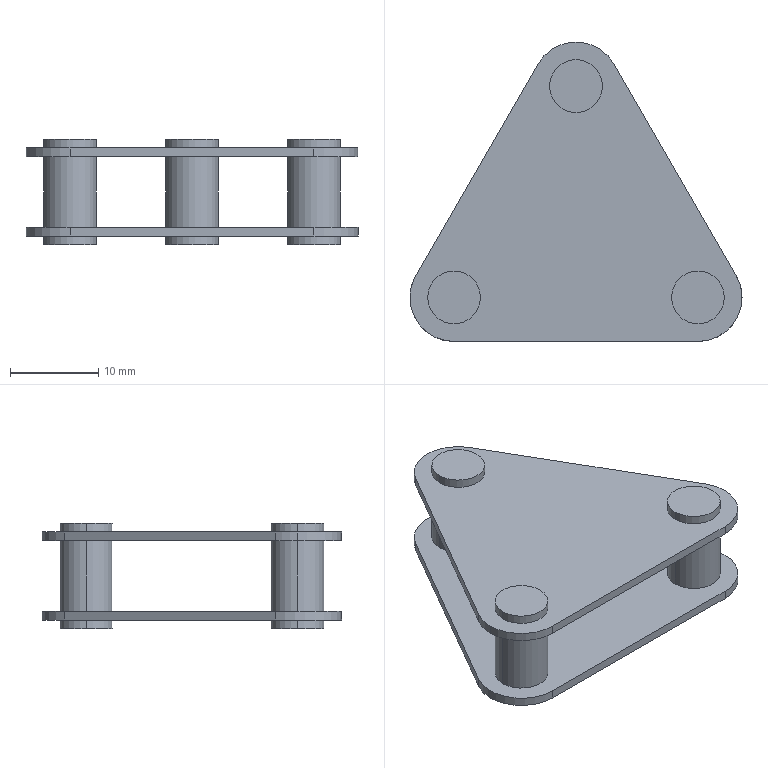Part | SolidWorks | features ICE 2, Extrusion 1, MirrorPattern 1 | 1 solid | 42 faces | box 37.679 x 33.971 x 12 mm | volume 2499 mm3 | cylinder 26 | plane 16 | commonest cylinder face diameters 6 x18 10 x8
STEP:
#1=CARTESIAN_POINT('',(-10.84,-7.99,2.));
#2=VERTEX_POINT('',#1);
#3=CARTESIAN_POINT('',(-16.84,-7.99,2.));
#4=VERTEX_POINT('',#3);
#5=CARTESIAN_POINT('',(-13.84,-7.99,2.));
#6=DIRECTION('',(0.,0.,1.));
#7=DIRECTION('',(1.,0.,0.));
#8=AXIS2_PLACEMENT_3D('',#5,#6,#7);
#9=CIRCLE('',#8,3.);
#10=EDGE_CURVE('',#2,#4,#9,.T.);
#11=ORIENTED_EDGE('',*,*,#10,.F.);
#12=CARTESIAN_POINT('',(-10.84,-7.99,1.));
#13=VERTEX_POINT('',#12);
#14=CARTESIAN_POINT('',(-10.84,-7.99,2.));
#15=DIRECTION('',(0.,0.,-1.));
#16=VECTOR('',#15,1000.);
#17=LINE('',#14,#16);
#18=EDGE_CURVE('',#2,#13,#17,.T.);
#19=ORIENTED_EDGE('',*,*,#18,.T.);
#20=CARTESIAN_POINT('',(-16.84,-7.99,1.));
#21=VERTEX_POINT('',#20);
#22=CARTESIAN_POINT('',(-13.84,-7.99,1.));
#23=DIRECTION('',(0.,0.,1.));
#24=DIRECTION('',(1.,0.,0.));
#25=AXIS2_PLACEMENT_3D('',#22,#23,#24);
#26=CIRCLE('',#25,3.);
#27=EDGE_CURVE('',#13,#21,#26,.T.);
#28=ORIENTED_EDGE('',*,*,#27,.T.);
#29=CARTESIAN_POINT('',(-16.84,-7.99,2.));
#30=DIRECTION('',(0.,0.,-1.));
#31=VECTOR('',#30,1000.);
#32=LINE('',#29,#31);
#33=EDGE_CURVE('',#4,#21,#32,.T.);
#34=ORIENTED_EDGE('',*,*,#33,.F.);
#35=EDGE_LOOP('',(#11,#19,#28,#34));
#36=FACE_OUTER_BOUND('',#35,.T.);
#37=CARTESIAN_POINT('',(-13.84,-7.99,2.));
#38=DIRECTION('',(0.,0.,-1.));
#39=DIRECTION('',(-1.,0.,0.));
#40=AXIS2_PLACEMENT_3D('',#37,#38,#39);
#41=CYLINDRICAL_SURFACE('',#40,3.);
#42=ADVANCED_FACE('',(#36),#41,.T.);
#43=CARTESIAN_POINT('',(16.84,-7.99,2.));
#44=VERTEX_POINT('',#43);
#45=CARTESIAN_POINT('',(10.84,-7.99,2.));
#46=VERTEX_POINT('',#45);
#47=CARTESIAN_POINT('',(13.84,-7.99,2.));
#48=DIRECTION('',(0.,0.,1.));
#49=DIRECTION('',(1.,0.,0.));
#50=AXIS2_PLACEMENT_3D('',#47,#48,#49);
#51=CIRCLE('',#50,3.);
#52=EDGE_CURVE('',#44,#46,#51,.T.);
#53=ORIENTED_EDGE('',*,*,#52,.F.);
#54=CARTESIAN_POINT('',(16.84,-7.99,1.));
#55=VERTEX_POINT('',#54);
#56=CARTESIAN_POINT('',(16.84,-7.99,2.));
#57=DIRECTION('',(0.,0.,-1.));
#58=VECTOR('',#57,1000.);
#59=LINE('',#56,#58);
#60=EDGE_CURVE('',#44,#55,#59,.T.);
#61=ORIENTED_EDGE('',*,*,#60,.T.);
#62=CARTESIAN_POINT('',(10.84,-7.99,1.));
#63=VERTEX_POINT('',#62);
#64=CARTESIAN_POINT('',(13.84,-7.99,1.));
#65=DIRECTION('',(0.,0.,1.));
#66=DIRECTION('',(1.,0.,0.));
#67=AXIS2_PLACEMENT_3D('',#64,#65,#66);
#68=CIRCLE('',#67,3.);
#69=EDGE_CURVE('',#55,#63,#68,.T.);
#70=ORIENTED_EDGE('',*,*,#69,.T.);
#71=CARTESIAN_POINT('',(10.84,-7.99,2.));
#72=DIRECTION('',(0.,0.,-1.));
#73=VECTOR('',#72,1000.);
#74=LINE('',#71,#73);
#75=EDGE_CURVE('',#46,#63,#74,.T.);
#76=ORIENTED_EDGE('',*,*,#75,.F.);
#77=EDGE_LOOP('',(#53,#61,#70,#76));
#78=FACE_OUTER_BOUND('',#77,.T.);
#79=CARTESIAN_POINT('',(13.84,-7.99,2.));
#80=DIRECTION('',(0.,0.,-1.));
#81=DIRECTION('',(-1.,0.,0.));
#82=AXIS2_PLACEMENT_3D('',#79,#80,#81);
#83=CYLINDRICAL_SURFACE('',#82,3.);
#84=ADVANCED_FACE('',(#78),#83,.T.);
#85=CARTESIAN_POINT('',(3.,15.981,2.));
#86=VERTEX_POINT('',#85);
#87=CARTESIAN_POINT('',(-3.,15.981,2.));
#88=VERTEX_POINT('',#87);
#89=CARTESIAN_POINT('',(0.,15.981,2.));
#90=DIRECTION('',(0.,0.,1.));
#91=DIRECTION('',(1.,0.,0.));
#92=AXIS2_PLACEMENT_3D('',#89,#90,#91);
#93=CIRCLE('',#92,3.);
#94=EDGE_CURVE('',#86,#88,#93,.T.);
#95=ORIENTED_EDGE('',*,*,#94,.F.);
#96=CARTESIAN_POINT('',(3.,15.981,1.));
#97=VERTEX_POINT('',#96);
#98=CARTESIAN_POINT('',(3.,15.981,2.));
#99=DIRECTION('',(0.,0.,-1.));
#100=VECTOR('',#99,1000.);
#101=LINE('',#98,#100);
#102=EDGE_CURVE('',#86,#97,#101,.T.);
#103=ORIENTED_EDGE('',*,*,#102,.T.);
#104=CARTESIAN_POINT('',(-3.,15.981,1.));
#105=VERTEX_POINT('',#104);
#106=CARTESIAN_POINT('',(0.,15.981,1.));
#107=DIRECTION('',(0.,0.,1.));
#108=DIRECTION('',(1.,0.,0.));
#109=AXIS2_PLACEMENT_3D('',#106,#107,#108);
#110=CIRCLE('',#109,3.);
#111=EDGE_CURVE('',#97,#105,#110,.T.);
#112=ORIENTED_EDGE('',*,*,#111,.T.);
#113=CARTESIAN_POINT('',(-3.,15.981,2.));
#114=DIRECTION('',(0.,0.,-1.));
#115=VECTOR('',#114,1000.);
#116=LINE('',#113,#115);
#117=EDGE_CURVE('',#88,#105,#116,.T.);
#118=ORIENTED_EDGE('',*,*,#117,.F.);
#119=EDGE_LOOP('',(#95,#103,#112,#118));
#120=FACE_OUTER_BOUND('',#119,.T.);
#121=CARTESIAN_POINT('',(0.,15.981,2.));
#122=DIRECTION('',(0.,0.,-1.));
#123=DIRECTION('',(-1.,0.,0.));
#124=AXIS2_PLACEMENT_3D('',#121,#122,#123);
#125=CYLINDRICAL_SURFACE('',#124,3.);
#126=ADVANCED_FACE('',(#120),#125,.T.);
#127=CARTESIAN_POINT('',(16.84,-7.99,-10.));
#128=VERTEX_POINT('',#127);
#129=CARTESIAN_POINT('',(10.84,-7.99,-10.));
#130=VERTEX_POINT('',#129);
#131=CARTESIAN_POINT('',(13.84,-7.99,-10.));
#132=DIRECTION('',(0.,0.,1.));
#133=DIRECTION('',(1.,0.,0.));
#134=AXIS2_PLACEMENT_3D('',#131,#132,#133);
#135=CIRCLE('',#134,3.);
#136=EDGE_CURVE('',#128,#130,#135,.T.);
#137=ORIENTED_EDGE('',*,*,#136,.T.);
#138=CARTESIAN_POINT('',(10.84,-7.99,-9.));
#139=VERTEX_POINT('',#138);
#140=CARTESIAN_POINT('',(10.84,-7.99,-10.));
#141=DIRECTION('',(0.,0.,1.));
#142=VECTOR('',#141,1000.);
#143=LINE('',#140,#142);
#144=EDGE_CURVE('',#130,#139,#143,.T.);
#145=ORIENTED_EDGE('',*,*,#144,.T.);
#146=CARTESIAN_POINT('',(16.84,-7.99,-9.));
#147=VERTEX_POINT('',#146);
#148=CARTESIAN_POINT('',(13.84,-7.99,-9.));
#149=DIRECTION('',(0.,0.,1.));
#150=DIRECTION('',(-1.,0.,0.));
#151=AXIS2_PLACEMENT_3D('',#148,#149,#150);
#152=CIRCLE('',#151,3.);
#153=EDGE_CURVE('',#147,#139,#152,.T.);
#154=ORIENTED_EDGE('',*,*,#153,.F.);
#155=CARTESIAN_POINT('',(16.84,-7.99,-10.));
#156=DIRECTION('',(0.,0.,1.));
#157=VECTOR('',#156,1000.);
#158=LINE('',#155,#157);
#159=EDGE_CURVE('',#128,#147,#158,.T.);
#160=ORIENTED_EDGE('',*,*,#159,.F.);
#161=EDGE_LOOP('',(#137,#145,#154,#160));
#162=FACE_OUTER_BOUND('',#161,.T.);
#163=CARTESIAN_POINT('',(13.84,-7.99,-10.));
#164=DIRECTION('',(0.,0.,1.));
#165=DIRECTION('',(1.,0.,0.));
#166=AXIS2_PLACEMENT_3D('',#163,#164,#165);
#167=CYLINDRICAL_SURFACE('',#166,3.);
#168=ADVANCED_FACE('',(#162),#167,.T.);
#169=CARTESIAN_POINT('',(-10.84,-7.99,-10.));
#170=VERTEX_POINT('',#169);
#171=CARTESIAN_POINT('',(-16.84,-7.99,-10.));
#172=VERTEX_POINT('',#171);
#173=CARTESIAN_POINT('',(-13.84,-7.99,-10.));
#174=DIRECTION('',(0.,0.,1.));
#175=DIRECTION('',(1.,0.,0.));
#176=AXIS2_PLACEMENT_3D('',#173,#174,#175);
#177=CIRCLE('',#176,3.);
#178=EDGE_CURVE('',#170,#172,#177,.T.);
#179=ORIENTED_EDGE('',*,*,#178,.T.);
#180=CARTESIAN_POINT('',(-16.84,-7.99,-9.));
#181=VERTEX_POINT('',#180);
#182=CARTESIAN_POINT('',(-16.84,-7.99,-10.));
#183=DIRECTION('',(0.,0.,1.));
#184=VECTOR('',#183,1000.);
#185=LINE('',#182,#184);
#186=EDGE_CURVE('',#172,#181,#185,.T.);
#187=ORIENTED_EDGE('',*,*,#186,.T.);
#188=CARTESIAN_POINT('',(-10.84,-7.99,-9.));
#189=VERTEX_POINT('',#188);
#190=CARTESIAN_POINT('',(-13.84,-7.99,-9.));
#191=DIRECTION('',(0.,0.,1.));
#192=DIRECTION('',(-1.,0.,0.));
#193=AXIS2_PLACEMENT_3D('',#190,#191,#192);
#194=CIRCLE('',#193,3.);
#195=EDGE_CURVE('',#189,#181,#194,.T.);
#196=ORIENTED_EDGE('',*,*,#195,.F.);
#197=CARTESIAN_POINT('',(-10.84,-7.99,-10.));
#198=DIRECTION('',(0.,0.,1.));
#199=VECTOR('',#198,1000.);
#200=LINE('',#197,#199);
#201=EDGE_CURVE('',#170,#189,#200,.T.);
#202=ORIENTED_EDGE('',*,*,#201,.F.);
#203=EDGE_LOOP('',(#179,#187,#196,#202));
#204=FACE_OUTER_BOUND('',#203,.T.);
#205=CARTESIAN_POINT('',(-13.84,-7.99,-10.));
#206=DIRECTION('',(0.,0.,1.));
#207=DIRECTION('',(1.,0.,0.));
#208=AXIS2_PLACEMENT_3D('',#205,#206,#207);
#209=CYLINDRICAL_SURFACE('',#208,3.);
#210=ADVANCED_FACE('',(#204),#209,.T.);
#211=CARTESIAN_POINT('',(3.,15.981,-10.));
#212=VERTEX_POINT('',#211);
#213=CARTESIAN_POINT('',(-3.,15.981,-10.));
#214=VERTEX_POINT('',#213);
#215=CARTESIAN_POINT('',(0.,15.981,-10.));
#216=DIRECTION('',(0.,0.,1.));
#217=DIRECTION('',(1.,0.,0.));
#218=AXIS2_PLACEMENT_3D('',#215,#216,#217);
#219=CIRCLE('',#218,3.);
#220=EDGE_CURVE('',#212,#214,#219,.T.);
#221=ORIENTED_EDGE('',*,*,#220,.T.);
#222=CARTESIAN_POINT('',(-3.,15.981,-9.));
#223=VERTEX_POINT('',#222);
#224=CARTESIAN_POINT('',(-3.,15.981,-10.));
#225=DIRECTION('',(0.,0.,1.));
#226=VECTOR('',#225,1000.);
#227=LINE('',#224,#226);
#228=EDGE_CURVE('',#214,#223,#227,.T.);
#229=ORIENTED_EDGE('',*,*,#228,.T.);
#230=CARTESIAN_POINT('',(3.,15.981,-9.));
#231=VERTEX_POINT('',#230);
#232=CARTESIAN_POINT('',(0.,15.981,-9.));
#233=DIRECTION('',(0.,0.,1.));
#234=DIRECTION('',(-1.,0.,0.));
#235=AXIS2_PLACEMENT_3D('',#232,#233,#234);
#236=CIRCLE('',#235,3.);
#237=EDGE_CURVE('',#231,#223,#236,.T.);
#238=ORIENTED_EDGE('',*,*,#237,.F.);
#239=CARTESIAN_POINT('',(3.,15.981,-10.));
#240=DIRECTION('',(0.,0.,1.));
#241=VECTOR('',#240,1000.);
#242=LINE('',#239,#241);
#243=EDGE_CURVE('',#212,#231,#242,.T.);
#244=ORIENTED_EDGE('',*,*,#243,.F.);
#245=EDGE_LOOP('',(#221,#229,#238,#244));
#246=FACE_OUTER_BOUND('',#245,.T.);
#247=CARTESIAN_POINT('',(0.,15.981,-10.));
#248=DIRECTION('',(0.,0.,1.));
#249=DIRECTION('',(1.,0.,0.));
#250=AXIS2_PLACEMENT_3D('',#247,#248,#249);
#251=CYLINDRICAL_SURFACE('',#250,3.);
#252=ADVANCED_FACE('',(#246),#251,.T.);
#253=CARTESIAN_POINT('',(13.84,-12.99,-9.));
#254=VERTEX_POINT('',#253);
#255=CARTESIAN_POINT('',(18.84,-7.99,-9.));
#256=VERTEX_POINT('',#255);
#257=CARTESIAN_POINT('',(13.84,-7.99,-9.));
#258=DIRECTION('',(0.,0.,1.));
#259=DIRECTION('',(1.,0.,0.));
#260=AXIS2_PLACEMENT_3D('',#257,#258,#259);
#261=CIRCLE('',#260,5.);
#262=EDGE_CURVE('',#254,#256,#261,.T.);
#263=ORIENTED_EDGE('',*,*,#262,.T.);
#264=CARTESIAN_POINT('',(18.84,-7.99,-8.));
#265=VERTEX_POINT('',#264);
#266=CARTESIAN_POINT('',(18.84,-7.99,-9.));
#267=DIRECTION('',(0.,0.,1.));
#268=VECTOR('',#267,1000.);
#269=LINE('',#266,#268);
#270=EDGE_CURVE('',#256,#265,#269,.T.);
#271=ORIENTED_EDGE('',*,*,#270,.T.);
#272=CARTESIAN_POINT('',(13.84,-12.99,-8.));
#273=VERTEX_POINT('',#272);
#274=CARTESIAN_POINT('',(13.84,-7.99,-8.));
#275=DIRECTION('',(0.,0.,1.));
#276=DIRECTION('',(1.,0.,0.));
#277=AXIS2_PLACEMENT_3D('',#274,#275,#276);
#278=CIRCLE('',#277,5.);
#279=EDGE_CURVE('',#273,#265,#278,.T.);
#280=ORIENTED_EDGE('',*,*,#279,.F.);
#281=CARTESIAN_POINT('',(13.84,-12.99,-9.));
#282=DIRECTION('',(0.,0.,1.));
#283=VECTOR('',#282,1000.);
#284=LINE('',#281,#283);
#285=EDGE_CURVE('',#254,#273,#284,.T.);
#286=ORIENTED_EDGE('',*,*,#285,.F.);
#287=EDGE_LOOP('',(#263,#271,#280,#286));
#288=FACE_OUTER_BOUND('',#287,.T.);
#289=CARTESIAN_POINT('',(13.84,-7.99,-9.));
#290=DIRECTION('',(0.,0.,1.));
#291=DIRECTION('',(1.,0.,0.));
#292=AXIS2_PLACEMENT_3D('',#289,#290,#291);
#293=CYLINDRICAL_SURFACE('',#292,5.);
#294=ADVANCED_FACE('',(#288),#293,.T.);
#295=CARTESIAN_POINT('',(-18.84,-7.99,1.));
#296=VERTEX_POINT('',#295);
#297=CARTESIAN_POINT('',(-13.84,-12.99,1.));
#298=VERTEX_POINT('',#297);
#299=CARTESIAN_POINT('',(-13.84,-7.99,1.));
#300=DIRECTION('',(0.,0.,1.));
#301=DIRECTION('',(-1.,0.,0.));
#302=AXIS2_PLACEMENT_3D('',#299,#300,#301);
#303=CIRCLE('',#302,5.);
#304=EDGE_CURVE('',#296,#298,#303,.T.);
#305=ORIENTED_EDGE('',*,*,#304,.F.);
#306=CARTESIAN_POINT('',(-18.84,-7.99,0.));
#307=VERTEX_POINT('',#306);
#308=CARTESIAN_POINT('',(-18.84,-7.99,1.));
#309=DIRECTION('',(0.,0.,-1.));
#310=VECTOR('',#309,1000.);
#311=LINE('',#308,#310);
#312=EDGE_CURVE('',#296,#307,#311,.T.);
#313=ORIENTED_EDGE('',*,*,#312,.T.);
#314=CARTESIAN_POINT('',(-13.84,-12.99,0.));
#315=VERTEX_POINT('',#314);
#316=CARTESIAN_POINT('',(-13.84,-7.99,0.));
#317=DIRECTION('',(0.,0.,1.));
#318=DIRECTION('',(-1.,0.,0.));
#319=AXIS2_PLACEMENT_3D('',#316,#317,#318);
#320=CIRCLE('',#319,5.);
#321=EDGE_CURVE('',#307,#315,#320,.T.);
#322=ORIENTED_EDGE('',*,*,#321,.T.);
#323=CARTESIAN_POINT('',(-13.84,-12.99,1.));
#324=DIRECTION('',(0.,0.,-1.));
#325=VECTOR('',#324,1000.);
#326=LINE('',#323,#325);
#327=EDGE_CURVE('',#298,#315,#326,.T.);
#328=ORIENTED_EDGE('',*,*,#327,.F.);
#329=EDGE_LOOP('',(#305,#313,#322,#328));
#330=FACE_OUTER_BOUND('',#329,.T.);
#331=CARTESIAN_POINT('',(-13.84,-7.99,1.));
#332=DIRECTION('',(0.,0.,-1.));
#333=DIRECTION('',(-1.,0.,0.));
#334=AXIS2_PLACEMENT_3D('',#331,#332,#333);
#335=CYLINDRICAL_SURFACE('',#334,5.);
#336=ADVANCED_FACE('',(#330),#335,.T.);
#337=CARTESIAN_POINT('',(3.,15.981,-8.));
#338=VERTEX_POINT('',#337);
#339=CARTESIAN_POINT('',(-3.,15.981,-8.));
#340=VERTEX_POINT('',#339);
#341=CARTESIAN_POINT('',(0.,15.981,-8.));
#342=DIRECTION('',(0.,0.,1.));
#343=DIRECTION('',(1.,0.,0.));
#344=AXIS2_PLACEMENT_3D('',#341,#342,#343);
#345=CIRCLE('',#344,3.);
#346=EDGE_CURVE('',#338,#340,#345,.T.);
#347=ORIENTED_EDGE('',*,*,#346,.T.);
#348=CARTESIAN_POINT('',(-3.,15.981,0.));
#349=VERTEX_POINT('',#348);
#350=CARTESIAN_POINT('',(-3.,15.981,-10.));
#351=DIRECTION('',(0.,0.,1.));
#352=VECTOR('',#351,1000.);
#353=LINE('',#350,#352);
#354=EDGE_CURVE('',#340,#349,#353,.T.);
#355=ORIENTED_EDGE('',*,*,#354,.T.);
#356=CARTESIAN_POINT('',(3.,15.981,0.));
#357=VERTEX_POINT('',#356);
#358=CARTESIAN_POINT('',(0.,15.981,0.));
#359=DIRECTION('',(0.,0.,1.));
#360=DIRECTION('',(1.,0.,0.));
#361=AXIS2_PLACEMENT_3D('',#358,#359,#360);
#362=CIRCLE('',#361,3.);
#363=EDGE_CURVE('',#357,#349,#362,.T.);
#364=ORIENTED_EDGE('',*,*,#363,.F.);
#365=CARTESIAN_POINT('',(3.,15.981,-10.));
#366=DIRECTION('',(0.,0.,1.));
#367=VECTOR('',#366,1000.);
#368=LINE('',#365,#367);
#369=EDGE_CURVE('',#338,#357,#368,.T.);
#370=ORIENTED_EDGE('',*,*,#369,.F.);
#371=EDGE_LOOP('',(#347,#355,#364,#370));
#372=FACE_OUTER_BOUND('',#371,.T.);
#373=CARTESIAN_POINT('',(0.,15.981,-10.));
#374=DIRECTION('',(0.,0.,1.));
#375=DIRECTION('',(1.,0.,0.));
#376=AXIS2_PLACEMENT_3D('',#373,#374,#375);
#377=CYLINDRICAL_SURFACE('',#376,3.);
#378=ADVANCED_FACE('',(#372),#377,.T.);
#379=CARTESIAN_POINT('',(-10.84,-7.99,-8.));
#380=VERTEX_POINT('',#379);
#381=CARTESIAN_POINT('',(-16.84,-7.99,-8.));
#382=VERTEX_POINT('',#381);
#383=CARTESIAN_POINT('',(-13.84,-7.99,-8.));
#384=DIRECTION('',(0.,0.,1.));
#385=DIRECTION('',(1.,0.,0.));
#386=AXIS2_PLACEMENT_3D('',#383,#384,#385);
#387=CIRCLE('',#386,3.);
#388=EDGE_CURVE('',#380,#382,#387,.T.);
#389=ORIENTED_EDGE('',*,*,#388,.T.);
#390=CARTESIAN_POINT('',(-16.84,-7.99,0.));
#391=VERTEX_POINT('',#390);
#392=CARTESIAN_POINT('',(-16.84,-7.99,-10.));
#393=DIRECTION('',(0.,0.,1.));
#394=VECTOR('',#393,1000.);
#395=LINE('',#392,#394);
#396=EDGE_CURVE('',#382,#391,#395,.T.);
#397=ORIENTED_EDGE('',*,*,#396,.T.);
#398=CARTESIAN_POINT('',(-10.84,-7.99,0.));
#399=VERTEX_POINT('',#398);
#400=CARTESIAN_POINT('',(-13.84,-7.99,0.));
#401=DIRECTION('',(0.,0.,1.));
#402=DIRECTION('',(1.,0.,0.));
#403=AXIS2_PLACEMENT_3D('',#400,#401,#402);
#404=CIRCLE('',#403,3.);
#405=EDGE_CURVE('',#399,#391,#404,.T.);
#406=ORIENTED_EDGE('',*,*,#405,.F.);
#407=CARTESIAN_POINT('',(-10.84,-7.99,-10.));
#408=DIRECTION('',(0.,0.,1.));
#409=VECTOR('',#408,1000.);
#410=LINE('',#407,#409);
#411=EDGE_CURVE('',#380,#399,#410,.T.);
#412=ORIENTED_EDGE('',*,*,#411,.F.);
#413=EDGE_LOOP('',(#389,#397,#406,#412));
#414=FACE_OUTER_BOUND('',#413,.T.);
#415=CARTESIAN_POINT('',(-13.84,-7.99,-10.));
#416=DIRECTION('',(0.,0.,1.));
#417=DIRECTION('',(1.,0.,0.));
#418=AXIS2_PLACEMENT_3D('',#415,#416,#417);
#419=CYLINDRICAL_SURFACE('',#418,3.);
#420=ADVANCED_FACE('',(#414),#419,.T.);
#421=CARTESIAN_POINT('',(16.84,-7.99,-8.));
#422=VERTEX_POINT('',#421);
#423=CARTESIAN_POINT('',(10.84,-7.99,-8.));
#424=VERTEX_POINT('',#423);
#425=CARTESIAN_POINT('',(13.84,-7.99,-8.));
#426=DIRECTION('',(0.,0.,1.));
#427=DIRECTION('',(1.,0.,0.));
#428=AXIS2_PLACEMENT_3D('',#425,#426,#427);
#429=CIRCLE('',#428,3.);
#430=EDGE_CURVE('',#422,#424,#429,.T.);
#431=ORIENTED_EDGE('',*,*,#430,.T.);
#432=CARTESIAN_POINT('',(10.84,-7.99,0.));
#433=VERTEX_POINT('',#432);
#434=CARTESIAN_POINT('',(10.84,-7.99,-10.));
#435=DIRECTION('',(0.,0.,1.));
#436=VECTOR('',#435,1000.);
#437=LINE('',#434,#436);
#438=EDGE_CURVE('',#424,#433,#437,.T.);
#439=ORIENTED_EDGE('',*,*,#438,.T.);
#440=CARTESIAN_POINT('',(16.84,-7.99,0.));
#441=VERTEX_POINT('',#440);
#442=CARTESIAN_POINT('',(13.84,-7.99,0.));
#443=DIRECTION('',(0.,0.,1.));
#444=DIRECTION('',(1.,0.,0.));
#445=AXIS2_PLACEMENT_3D('',#442,#443,#444);
#446=CIRCLE('',#445,3.);
#447=EDGE_CURVE('',#441,#433,#446,.T.);
#448=ORIENTED_EDGE('',*,*,#447,.F.);
#449=CARTESIAN_POINT('',(16.84,-7.99,-10.));
#450=DIRECTION('',(0.,0.,1.));
#451=VECTOR('',#450,1000.);
#452=LINE('',#449,#451);
#453=EDGE_CURVE('',#422,#441,#452,.T.);
#454=ORIENTED_EDGE('',*,*,#453,.F.);
#455=EDGE_LOOP('',(#431,#439,#448,#454));
#456=FACE_OUTER_BOUND('',#455,.T.);
#457=CARTESIAN_POINT('',(13.84,-7.99,-10.));
#458=DIRECTION('',(0.,0.,1.));
#459=DIRECTION('',(1.,0.,0.));
#460=AXIS2_PLACEMENT_3D('',#457,#458,#459);
#461=CYLINDRICAL_SURFACE('',#460,3.);
#462=ADVANCED_FACE('',(#456),#461,.T.);
#463=ORIENTED_EDGE('',*,*,#438,.F.);
#464=CARTESIAN_POINT('',(13.84,-7.99,-8.));
#465=DIRECTION('',(0.,0.,1.));
#466=DIRECTION('',(1.,0.,0.));
#467=AXIS2_PLACEMENT_3D('',#464,#465,#466);
#468=CIRCLE('',#467,3.);
#469=EDGE_CURVE('',#424,#422,#468,.T.);
#470=ORIENTED_EDGE('',*,*,#469,.T.);
#471=ORIENTED_EDGE('',*,*,#453,.T.);
#472=CARTESIAN_POINT('',(13.84,-7.99,0.));
#473=DIRECTION('',(0.,0.,1.));
#474=DIRECTION('',(1.,0.,0.));
#475=AXIS2_PLACEMENT_3D('',#472,#473,#474);
#476=CIRCLE('',#475,3.);
#477=EDGE_CURVE('',#433,#441,#476,.T.);
#478=ORIENTED_EDGE('',*,*,#477,.F.);
#479=EDGE_LOOP('',(#463,#470,#471,#478));
#480=FACE_OUTER_BOUND('',#479,.T.);
#481=CARTESIAN_POINT('',(13.84,-7.99,-10.));
#482=DIRECTION('',(0.,0.,1.));
#483=DIRECTION('',(1.,0.,0.));
#484=AXIS2_PLACEMENT_3D('',#481,#482,#483);
#485=CYLINDRICAL_SURFACE('',#484,3.);
#486=ADVANCED_FACE('',(#480),#485,.T.);
#487=ORIENTED_EDGE('',*,*,#396,.F.);
#488=CARTESIAN_POINT('',(-13.84,-7.99,-8.));
#489=DIRECTION('',(0.,0.,1.));
#490=DIRECTION('',(1.,0.,0.));
#491=AXIS2_PLACEMENT_3D('',#488,#489,#490);
#492=CIRCLE('',#491,3.);
#493=EDGE_CURVE('',#382,#380,#492,.T.);
#494=ORIENTED_EDGE('',*,*,#493,.T.);
#495=ORIENTED_EDGE('',*,*,#411,.T.);
#496=CARTESIAN_POINT('',(-13.84,-7.99,0.));
#497=DIRECTION('',(0.,0.,1.));
#498=DIRECTION('',(1.,0.,0.));
#499=AXIS2_PLACEMENT_3D('',#496,#497,#498);
#500=CIRCLE('',#499,3.);
#501=EDGE_CURVE('',#391,#399,#500,.T.);
#502=ORIENTED_EDGE('',*,*,#501,.F.);
#503=EDGE_LOOP('',(#487,#494,#495,#502));
#504=FACE_OUTER_BOUND('',#503,.T.);
#505=CARTESIAN_POINT('',(-13.84,-7.99,-10.));
#506=DIRECTION('',(0.,0.,1.));
#507=DIRECTION('',(1.,0.,0.));
#508=AXIS2_PLACEMENT_3D('',#505,#506,#507);
#509=CYLINDRICAL_SURFACE('',#508,3.);
#510=ADVANCED_FACE('',(#504),#509,.T.);
#511=ORIENTED_EDGE('',*,*,#354,.F.);
#512=CARTESIAN_POINT('',(0.,15.981,-8.));
#513=DIRECTION('',(0.,0.,1.));
#514=DIRECTION('',(1.,0.,0.));
#515=AXIS2_PLACEMENT_3D('',#512,#513,#514);
#516=CIRCLE('',#515,3.);
#517=EDGE_CURVE('',#340,#338,#516,.T.);
#518=ORIENTED_EDGE('',*,*,#517,.T.);
#519=ORIENTED_EDGE('',*,*,#369,.T.);
#520=CARTESIAN_POINT('',(0.,15.981,0.));
#521=DIRECTION('',(0.,0.,1.));
#522=DIRECTION('',(1.,0.,0.));
#523=AXIS2_PLACEMENT_3D('',#520,#521,#522);
#524=CIRCLE('',#523,3.);
#525=EDGE_CURVE('',#349,#357,#524,.T.);
#526=ORIENTED_EDGE('',*,*,#525,.F.);
#527=EDGE_LOOP('',(#511,#518,#519,#526));
#528=FACE_OUTER_BOUND('',#527,.T.);
#529=CARTESIAN_POINT('',(0.,15.981,-10.));
#530=DIRECTION('',(0.,0.,1.));
#531=DIRECTION('',(1.,0.,0.));
#532=AXIS2_PLACEMENT_3D('',#529,#530,#531);
#533=CYLINDRICAL_SURFACE('',#532,3.);
#534=ADVANCED_FACE('',(#528),#533,.T.);
#535=CARTESIAN_POINT('',(-13.84,-7.99,1.));
#536=DIRECTION('',(0.,0.,1.));
#537=DIRECTION('',(1.,0.,0.));
#538=AXIS2_PLACEMENT_3D('',#535,#536,#537);
#539=CIRCLE('',#538,3.);
#540=EDGE_CURVE('',#21,#13,#539,.T.);
#541=ORIENTED_EDGE('',*,*,#540,.F.);
#542=ORIENTED_EDGE('',*,*,#27,.F.);
#543=EDGE_LOOP('',(#541,#542));
#544=FACE_BOUND('',#543,.T.);
#545=CARTESIAN_POINT('',(13.84,-7.99,1.));
#546=DIRECTION('',(0.,0.,1.));
#547=DIRECTION('',(1.,0.,0.));
#548=AXIS2_PLACEMENT_3D('',#545,#546,#547);
#549=CIRCLE('',#548,3.);
#550=EDGE_CURVE('',#63,#55,#549,.T.);
#551=ORIENTED_EDGE('',*,*,#550,.F.);
#552=ORIENTED_EDGE('',*,*,#69,.F.);
#553=EDGE_LOOP('',(#551,#552));
#554=FACE_BOUND('',#553,.T.);
#555=CARTESIAN_POINT('',(0.,15.981,1.));
#556=DIRECTION('',(0.,0.,1.));
#557=DIRECTION('',(1.,0.,0.));
#558=AXIS2_PLACEMENT_3D('',#555,#556,#557);
#559=CIRCLE('',#558,3.);
#560=EDGE_CURVE('',#105,#97,#559,.T.);
#561=ORIENTED_EDGE('',*,*,#560,.F.);
#562=ORIENTED_EDGE('',*,*,#111,.F.);
#563=EDGE_LOOP('',(#561,#562));
#564=FACE_BOUND('',#563,.T.);
#565=CARTESIAN_POINT('',(13.84,-12.99,1.));
#566=VERTEX_POINT('',#565);
#567=CARTESIAN_POINT('',(18.17,-5.49,1.));
#568=VERTEX_POINT('',#567);
#569=CARTESIAN_POINT('',(13.84,-7.99,1.));
#570=DIRECTION('',(0.,0.,1.));
#571=DIRECTION('',(1.,0.,0.));
#572=AXIS2_PLACEMENT_3D('',#569,#570,#571);
#573=CIRCLE('',#572,5.);
#574=EDGE_CURVE('',#566,#568,#573,.T.);
#575=ORIENTED_EDGE('',*,*,#574,.T.);
#576=CARTESIAN_POINT('',(4.33,18.481,1.));
#577=VERTEX_POINT('',#576);
#578=CARTESIAN_POINT('',(18.17,-5.49,1.));
#579=DIRECTION('',(-0.5,0.866,0.));
#580=VECTOR('',#579,1000.);
#581=LINE('',#578,#580);
#582=EDGE_CURVE('',#568,#577,#581,.T.);
#583=ORIENTED_EDGE('',*,*,#582,.T.);
#584=CARTESIAN_POINT('',(-4.33,18.481,1.));
#585=VERTEX_POINT('',#584);
#586=CARTESIAN_POINT('',(0.,15.981,1.));
#587=DIRECTION('',(0.,0.,1.));
#588=DIRECTION('',(1.,0.,0.));
#589=AXIS2_PLACEMENT_3D('',#586,#587,#588);
#590=CIRCLE('',#589,5.);
#591=EDGE_CURVE('',#577,#585,#590,.T.);
#592=ORIENTED_EDGE('',*,*,#591,.T.);
#593=CARTESIAN_POINT('',(-18.17,-5.49,1.));
#594=VERTEX_POINT('',#593);
#595=CARTESIAN_POINT('',(-4.33,18.481,1.));
#596=DIRECTION('',(-0.5,-0.866,0.));
#597=VECTOR('',#596,1000.);
#598=LINE('',#595,#597);
#599=EDGE_CURVE('',#585,#594,#598,.T.);
#600=ORIENTED_EDGE('',*,*,#599,.T.);
#601=CARTESIAN_POINT('',(-13.84,-7.99,1.));
#602=DIRECTION('',(0.,0.,1.));
#603=DIRECTION('',(-1.,0.,0.));
#604=AXIS2_PLACEMENT_3D('',#601,#602,#603);
#605=CIRCLE('',#604,5.);
#606=EDGE_CURVE('',#594,#296,#605,.T.);
#607=ORIENTED_EDGE('',*,*,#606,.T.);
#608=ORIENTED_EDGE('',*,*,#304,.T.);
#609=CARTESIAN_POINT('',(-13.84,-12.99,1.));
#610=DIRECTION('',(1.,0.,0.));
#611=VECTOR('',#610,1000.);
#612=LINE('',#609,#611);
#613=EDGE_CURVE('',#298,#566,#612,.T.);
#614=ORIENTED_EDGE('',*,*,#613,.T.);
#615=EDGE_LOOP('',(#575,#583,#592,#600,#607,#608,#614));
#616=FACE_OUTER_BOUND('',#615,.T.);
#617=CARTESIAN_POINT('',(13.84,-7.99,1.));
#618=DIRECTION('',(0.,0.,1.));
#619=DIRECTION('',(1.,0.,0.));
#620=AXIS2_PLACEMENT_3D('',#617,#618,#619);
#621=PLANE('',#620);
#622=ADVANCED_FACE('',(#544,#554,#564,#616),#621,.T.);
#623=CARTESIAN_POINT('',(13.84,-12.99,0.));
#624=VERTEX_POINT('',#623);
#625=CARTESIAN_POINT('',(18.17,-5.49,0.));
#626=VERTEX_POINT('',#625);
#627=CARTESIAN_POINT('',(13.84,-7.99,0.));
#628=DIRECTION('',(0.,0.,1.));
#629=DIRECTION('',(1.,0.,0.));
#630=AXIS2_PLACEMENT_3D('',#627,#628,#629);
#631=CIRCLE('',#630,5.);
#632=EDGE_CURVE('',#624,#626,#631,.T.);
#633=ORIENTED_EDGE('',*,*,#632,.F.);
#634=CARTESIAN_POINT('',(-13.84,-12.99,0.));
#635=DIRECTION('',(1.,0.,0.));
#636=VECTOR('',#635,1000.);
#637=LINE('',#634,#636);
#638=EDGE_CURVE('',#315,#624,#637,.T.);
#639=ORIENTED_EDGE('',*,*,#638,.F.);
#640=ORIENTED_EDGE('',*,*,#321,.F.);
#641=CARTESIAN_POINT('',(-18.17,-5.49,0.));
#642=VERTEX_POINT('',#641);
#643=CARTESIAN_POINT('',(-13.84,-7.99,0.));
#644=DIRECTION('',(0.,0.,1.));
#645=DIRECTION('',(-1.,0.,0.));
#646=AXIS2_PLACEMENT_3D('',#643,#644,#645);
#647=CIRCLE('',#646,5.);
#648=EDGE_CURVE('',#642,#307,#647,.T.);
#649=ORIENTED_EDGE('',*,*,#648,.F.);
#650=CARTESIAN_POINT('',(-4.33,18.481,0.));
#651=VERTEX_POINT('',#650);
#652=CARTESIAN_POINT('',(-4.33,18.481,0.));
#653=DIRECTION('',(-0.5,-0.866,0.));
#654=VECTOR('',#653,1000.);
#655=LINE('',#652,#654);
#656=EDGE_CURVE('',#651,#642,#655,.T.);
#657=ORIENTED_EDGE('',*,*,#656,.F.);
#658=CARTESIAN_POINT('',(4.33,18.481,0.));
#659=VERTEX_POINT('',#658);
#660=CARTESIAN_POINT('',(0.,15.981,0.));
#661=DIRECTION('',(0.,0.,1.));
#662=DIRECTION('',(1.,0.,0.));
#663=AXIS2_PLACEMENT_3D('',#660,#661,#662);
#664=CIRCLE('',#663,5.);
#665=EDGE_CURVE('',#659,#651,#664,.T.);
#666=ORIENTED_EDGE('',*,*,#665,.F.);
#667=CARTESIAN_POINT('',(18.17,-5.49,0.));
#668=DIRECTION('',(-0.5,0.866,0.));
#669=VECTOR('',#668,1000.);
#670=LINE('',#667,#669);
#671=EDGE_CURVE('',#626,#659,#670,.T.);
#672=ORIENTED_EDGE('',*,*,#671,.F.);
#673=EDGE_LOOP('',(#633,#639,#640,#649,#657,#666,#672));
#674=FACE_OUTER_BOUND('',#673,.T.);
#675=ORIENTED_EDGE('',*,*,#363,.T.);
#676=ORIENTED_EDGE('',*,*,#525,.T.);
#677=EDGE_LOOP('',(#675,#676));
#678=FACE_BOUND('',#677,.T.);
#679=ORIENTED_EDGE('',*,*,#447,.T.);
#680=ORIENTED_EDGE('',*,*,#477,.T.);
#681=EDGE_LOOP('',(#679,#680));
#682=FACE_BOUND('',#681,.T.);
#683=ORIENTED_EDGE('',*,*,#405,.T.);
#684=ORIENTED_EDGE('',*,*,#501,.T.);
#685=EDGE_LOOP('',(#683,#684));
#686=FACE_BOUND('',#685,.T.);
#687=CARTESIAN_POINT('',(13.84,-7.99,0.));
#688=DIRECTION('',(0.,0.,1.));
#689=DIRECTION('',(1.,0.,0.));
#690=AXIS2_PLACEMENT_3D('',#687,#688,#689);
#691=PLANE('',#690);
#692=ADVANCED_FACE('',(#674,#678,#682,#686),#691,.F.);
#693=ORIENTED_EDGE('',*,*,#632,.T.);
#694=CARTESIAN_POINT('',(18.17,-5.49,1.));
#695=DIRECTION('',(0.,0.,-1.));
#696=VECTOR('',#695,1000.);
#697=LINE('',#694,#696);
#698=EDGE_CURVE('',#568,#626,#697,.T.);
#699=ORIENTED_EDGE('',*,*,#698,.F.);
#700=ORIENTED_EDGE('',*,*,#574,.F.);
#701=CARTESIAN_POINT('',(13.84,-12.99,1.));
#702=DIRECTION('',(0.,0.,-1.));
#703=VECTOR('',#702,1000.);
#704=LINE('',#701,#703);
#705=EDGE_CURVE('',#566,#624,#704,.T.);
#706=ORIENTED_EDGE('',*,*,#705,.T.);
#707=EDGE_LOOP('',(#693,#699,#700,#706));
#708=FACE_OUTER_BOUND('',#707,.T.);
#709=CARTESIAN_POINT('',(13.84,-7.99,1.));
#710=DIRECTION('',(0.,0.,-1.));
#711=DIRECTION('',(-1.,0.,0.));
#712=AXIS2_PLACEMENT_3D('',#709,#710,#711);
#713=CYLINDRICAL_SURFACE('',#712,5.);
#714=ADVANCED_FACE('',(#708),#713,.T.);
#715=ORIENTED_EDGE('',*,*,#671,.T.);
#716=CARTESIAN_POINT('',(4.33,18.481,1.));
#717=DIRECTION('',(0.,0.,-1.));
#718=VECTOR('',#717,1000.);
#719=LINE('',#716,#718);
#720=EDGE_CURVE('',#577,#659,#719,.T.);
#721=ORIENTED_EDGE('',*,*,#720,.F.);
#722=ORIENTED_EDGE('',*,*,#582,.F.);
#723=ORIENTED_EDGE('',*,*,#698,.T.);
#724=EDGE_LOOP('',(#715,#721,#722,#723));
#725=FACE_OUTER_BOUND('',#724,.T.);
#726=CARTESIAN_POINT('',(18.17,-5.49,1.));
#727=DIRECTION('',(-0.866,-0.5,0.));
#728=DIRECTION('',(0.5,-0.866,0.));
#729=AXIS2_PLACEMENT_3D('',#726,#727,#728);
#730=PLANE('',#729);
#731=ADVANCED_FACE('',(#725),#730,.F.);
#732=ORIENTED_EDGE('',*,*,#665,.T.);
#733=CARTESIAN_POINT('',(-4.33,18.481,1.));
#734=DIRECTION('',(0.,0.,-1.));
#735=VECTOR('',#734,1000.);
#736=LINE('',#733,#735);
#737=EDGE_CURVE('',#585,#651,#736,.T.);
#738=ORIENTED_EDGE('',*,*,#737,.F.);
#739=ORIENTED_EDGE('',*,*,#591,.F.);
#740=ORIENTED_EDGE('',*,*,#720,.T.);
#741=EDGE_LOOP('',(#732,#738,#739,#740));
#742=FACE_OUTER_BOUND('',#741,.T.);
#743=CARTESIAN_POINT('',(0.,15.981,1.));
#744=DIRECTION('',(0.,0.,-1.));
#745=DIRECTION('',(-1.,0.,0.));
#746=AXIS2_PLACEMENT_3D('',#743,#744,#745);
#747=CYLINDRICAL_SURFACE('',#746,5.);
#748=ADVANCED_FACE('',(#742),#747,.T.);
#749=ORIENTED_EDGE('',*,*,#656,.T.);
#750=CARTESIAN_POINT('',(-18.17,-5.49,1.));
#751=DIRECTION('',(0.,0.,-1.));
#752=VECTOR('',#751,1000.);
#753=LINE('',#750,#752);
#754=EDGE_CURVE('',#594,#642,#753,.T.);
#755=ORIENTED_EDGE('',*,*,#754,.F.);
#756=ORIENTED_EDGE('',*,*,#599,.F.);
#757=ORIENTED_EDGE('',*,*,#737,.T.);
#758=EDGE_LOOP('',(#749,#755,#756,#757));
#759=FACE_OUTER_BOUND('',#758,.T.);
#760=CARTESIAN_POINT('',(-4.33,18.481,1.));
#761=DIRECTION('',(0.866,-0.5,0.));
#762=DIRECTION('',(0.5,0.866,0.));
#763=AXIS2_PLACEMENT_3D('',#760,#761,#762);
#764=PLANE('',#763);
#765=ADVANCED_FACE('',(#759),#764,.F.);
#766=ORIENTED_EDGE('',*,*,#312,.F.);
#767=ORIENTED_EDGE('',*,*,#606,.F.);
#768=ORIENTED_EDGE('',*,*,#754,.T.);
#769=ORIENTED_EDGE('',*,*,#648,.T.);
#770=EDGE_LOOP('',(#766,#767,#768,#769));
#771=FACE_OUTER_BOUND('',#770,.T.);
#772=CARTESIAN_POINT('',(-13.84,-7.99,1.));
#773=DIRECTION('',(0.,0.,-1.));
#774=DIRECTION('',(-1.,0.,0.));
#775=AXIS2_PLACEMENT_3D('',#772,#773,#774);
#776=CYLINDRICAL_SURFACE('',#775,5.);
#777=ADVANCED_FACE('',(#771),#776,.T.);
#778=ORIENTED_EDGE('',*,*,#638,.T.);
#779=ORIENTED_EDGE('',*,*,#705,.F.);
#780=ORIENTED_EDGE('',*,*,#613,.F.);
#781=ORIENTED_EDGE('',*,*,#327,.T.);
#782=EDGE_LOOP('',(#778,#779,#780,#781));
#783=FACE_OUTER_BOUND('',#782,.T.);
#784=CARTESIAN_POINT('',(-13.84,-12.99,1.));
#785=DIRECTION('',(0.,1.,0.));
#786=DIRECTION('',(0.,0.,1.));
#787=AXIS2_PLACEMENT_3D('',#784,#785,#786);
#788=PLANE('',#787);
#789=ADVANCED_FACE('',(#783),#788,.F.);
#790=ORIENTED_EDGE('',*,*,#270,.F.);
#791=CARTESIAN_POINT('',(18.17,-5.49,-9.));
#792=VERTEX_POINT('',#791);
#793=CARTESIAN_POINT('',(13.84,-7.99,-9.));
#794=DIRECTION('',(0.,0.,1.));
#795=DIRECTION('',(1.,0.,0.));
#796=AXIS2_PLACEMENT_3D('',#793,#794,#795);
#797=CIRCLE('',#796,5.);
#798=EDGE_CURVE('',#256,#792,#797,.T.);
#799=ORIENTED_EDGE('',*,*,#798,.T.);
#800=CARTESIAN_POINT('',(18.17,-5.49,-8.));
#801=VERTEX_POINT('',#800);
#802=CARTESIAN_POINT('',(18.17,-5.49,-9.));
#803=DIRECTION('',(0.,0.,1.));
#804=VECTOR('',#803,1000.);
#805=LINE('',#802,#804);
#806=EDGE_CURVE('',#792,#801,#805,.T.);
#807=ORIENTED_EDGE('',*,*,#806,.T.);
#808=CARTESIAN_POINT('',(13.84,-7.99,-8.));
#809=DIRECTION('',(0.,0.,1.));
#810=DIRECTION('',(1.,0.,0.));
#811=AXIS2_PLACEMENT_3D('',#808,#809,#810);
#812=CIRCLE('',#811,5.);
#813=EDGE_CURVE('',#265,#801,#812,.T.);
#814=ORIENTED_EDGE('',*,*,#813,.F.);
#815=EDGE_LOOP('',(#790,#799,#807,#814));
#816=FACE_OUTER_BOUND('',#815,.T.);
#817=CARTESIAN_POINT('',(13.84,-7.99,-9.));
#818=DIRECTION('',(0.,0.,1.));
#819=DIRECTION('',(1.,0.,0.));
#820=AXIS2_PLACEMENT_3D('',#817,#818,#819);
#821=CYLINDRICAL_SURFACE('',#820,5.);
#822=ADVANCED_FACE('',(#816),#821,.T.);
#823=CARTESIAN_POINT('',(-13.84,-12.99,-8.));
#824=VERTEX_POINT('',#823);
#825=CARTESIAN_POINT('',(-13.84,-12.99,-8.));
#826=DIRECTION('',(1.,0.,0.));
#827=VECTOR('',#826,1000.);
#828=LINE('',#825,#827);
#829=EDGE_CURVE('',#824,#273,#828,.T.);
#830=ORIENTED_EDGE('',*,*,#829,.F.);
#831=CARTESIAN_POINT('',(-13.84,-12.99,-9.));
#832=VERTEX_POINT('',#831);
#833=CARTESIAN_POINT('',(-13.84,-12.99,-9.));
#834=DIRECTION('',(0.,0.,1.));
#835=VECTOR('',#834,1000.);
#836=LINE('',#833,#835);
#837=EDGE_CURVE('',#832,#824,#836,.T.);
#838=ORIENTED_EDGE('',*,*,#837,.F.);
#839=CARTESIAN_POINT('',(-13.84,-12.99,-9.));
#840=DIRECTION('',(1.,0.,0.));
#841=VECTOR('',#840,1000.);
#842=LINE('',#839,#841);
#843=EDGE_CURVE('',#832,#254,#842,.T.);
#844=ORIENTED_EDGE('',*,*,#843,.T.);
#845=ORIENTED_EDGE('',*,*,#285,.T.);
#846=EDGE_LOOP('',(#830,#838,#844,#845));
#847=FACE_OUTER_BOUND('',#846,.T.);
#848=CARTESIAN_POINT('',(-13.84,-12.99,-9.));
#849=DIRECTION('',(0.,-1.,0.));
#850=DIRECTION('',(0.,0.,-1.));
#851=AXIS2_PLACEMENT_3D('',#848,#849,#850);
#852=PLANE('',#851);
#853=ADVANCED_FACE('',(#847),#852,.T.);
#854=CARTESIAN_POINT('',(-18.17,-5.49,-8.));
#855=VERTEX_POINT('',#854);
#856=CARTESIAN_POINT('',(-13.84,-7.99,-8.));
#857=DIRECTION('',(0.,0.,1.));
#858=DIRECTION('',(-1.,0.,0.));
#859=AXIS2_PLACEMENT_3D('',#856,#857,#858);
#860=CIRCLE('',#859,5.);
#861=EDGE_CURVE('',#855,#824,#860,.T.);
#862=ORIENTED_EDGE('',*,*,#861,.F.);
#863=CARTESIAN_POINT('',(-18.17,-5.49,-9.));
#864=VERTEX_POINT('',#863);
#865=CARTESIAN_POINT('',(-18.17,-5.49,-9.));
#866=DIRECTION('',(0.,0.,1.));
#867=VECTOR('',#866,1000.);
#868=LINE('',#865,#867);
#869=EDGE_CURVE('',#864,#855,#868,.T.);
#870=ORIENTED_EDGE('',*,*,#869,.F.);
#871=CARTESIAN_POINT('',(-13.84,-7.99,-9.));
#872=DIRECTION('',(0.,0.,1.));
#873=DIRECTION('',(-1.,0.,0.));
#874=AXIS2_PLACEMENT_3D('',#871,#872,#873);
#875=CIRCLE('',#874,5.);
#876=EDGE_CURVE('',#864,#832,#875,.T.);
#877=ORIENTED_EDGE('',*,*,#876,.T.);
#878=ORIENTED_EDGE('',*,*,#837,.T.);
#879=EDGE_LOOP('',(#862,#870,#877,#878));
#880=FACE_OUTER_BOUND('',#879,.T.);
#881=CARTESIAN_POINT('',(-13.84,-7.99,-9.));
#882=DIRECTION('',(0.,0.,1.));
#883=DIRECTION('',(1.,0.,0.));
#884=AXIS2_PLACEMENT_3D('',#881,#882,#883);
#885=CYLINDRICAL_SURFACE('',#884,5.);
#886=ADVANCED_FACE('',(#880),#885,.T.);
#887=CARTESIAN_POINT('',(-4.33,18.481,-8.));
#888=VERTEX_POINT('',#887);
#889=CARTESIAN_POINT('',(-4.33,18.481,-8.));
#890=DIRECTION('',(-0.5,-0.866,0.));
#891=VECTOR('',#890,1000.);
#892=LINE('',#889,#891);
#893=EDGE_CURVE('',#888,#855,#892,.T.);
#894=ORIENTED_EDGE('',*,*,#893,.F.);
#895=CARTESIAN_POINT('',(-4.33,18.481,-9.));
#896=VERTEX_POINT('',#895);
#897=CARTESIAN_POINT('',(-4.33,18.481,-9.));
#898=DIRECTION('',(0.,0.,1.));
#899=VECTOR('',#898,1000.);
#900=LINE('',#897,#899);
#901=EDGE_CURVE('',#896,#888,#900,.T.);
#902=ORIENTED_EDGE('',*,*,#901,.F.);
#903=CARTESIAN_POINT('',(-4.33,18.481,-9.));
#904=DIRECTION('',(-0.5,-0.866,0.));
#905=VECTOR('',#904,1000.);
#906=LINE('',#903,#905);
#907=EDGE_CURVE('',#896,#864,#906,.T.);
#908=ORIENTED_EDGE('',*,*,#907,.T.);
#909=ORIENTED_EDGE('',*,*,#869,.T.);
#910=EDGE_LOOP('',(#894,#902,#908,#909));
#911=FACE_OUTER_BOUND('',#910,.T.);
#912=CARTESIAN_POINT('',(-4.33,18.481,-9.));
#913=DIRECTION('',(-0.866,0.5,0.));
#914=DIRECTION('',(-0.5,-0.866,0.));
#915=AXIS2_PLACEMENT_3D('',#912,#913,#914);
#916=PLANE('',#915);
#917=ADVANCED_FACE('',(#911),#916,.T.);
#918=CARTESIAN_POINT('',(4.33,18.481,-8.));
#919=VERTEX_POINT('',#918);
#920=CARTESIAN_POINT('',(0.,15.981,-8.));
#921=DIRECTION('',(0.,0.,1.));
#922=DIRECTION('',(1.,0.,0.));
#923=AXIS2_PLACEMENT_3D('',#920,#921,#922);
#924=CIRCLE('',#923,5.);
#925=EDGE_CURVE('',#919,#888,#924,.T.);
#926=ORIENTED_EDGE('',*,*,#925,.F.);
#927=CARTESIAN_POINT('',(4.33,18.481,-9.));
#928=VERTEX_POINT('',#927);
#929=CARTESIAN_POINT('',(4.33,18.481,-9.));
#930=DIRECTION('',(0.,0.,1.));
#931=VECTOR('',#930,1000.);
#932=LINE('',#929,#931);
#933=EDGE_CURVE('',#928,#919,#932,.T.);
#934=ORIENTED_EDGE('',*,*,#933,.F.);
#935=CARTESIAN_POINT('',(0.,15.981,-9.));
#936=DIRECTION('',(0.,0.,1.));
#937=DIRECTION('',(1.,0.,0.));
#938=AXIS2_PLACEMENT_3D('',#935,#936,#937);
#939=CIRCLE('',#938,5.);
#940=EDGE_CURVE('',#928,#896,#939,.T.);
#941=ORIENTED_EDGE('',*,*,#940,.T.);
#942=ORIENTED_EDGE('',*,*,#901,.T.);
#943=EDGE_LOOP('',(#926,#934,#941,#942));
#944=FACE_OUTER_BOUND('',#943,.T.);
#945=CARTESIAN_POINT('',(0.,15.981,-9.));
#946=DIRECTION('',(0.,0.,1.));
#947=DIRECTION('',(1.,0.,0.));
#948=AXIS2_PLACEMENT_3D('',#945,#946,#947);
#949=CYLINDRICAL_SURFACE('',#948,5.);
#950=ADVANCED_FACE('',(#944),#949,.T.);
#951=CARTESIAN_POINT('',(18.17,-5.49,-8.));
#952=DIRECTION('',(-0.5,0.866,0.));
#953=VECTOR('',#952,1000.);
#954=LINE('',#951,#953);
#955=EDGE_CURVE('',#801,#919,#954,.T.);
#956=ORIENTED_EDGE('',*,*,#955,.F.);
#957=ORIENTED_EDGE('',*,*,#806,.F.);
#958=CARTESIAN_POINT('',(18.17,-5.49,-9.));
#959=DIRECTION('',(-0.5,0.866,0.));
#960=VECTOR('',#959,1000.);
#961=LINE('',#958,#960);
#962=EDGE_CURVE('',#792,#928,#961,.T.);
#963=ORIENTED_EDGE('',*,*,#962,.T.);
#964=ORIENTED_EDGE('',*,*,#933,.T.);
#965=EDGE_LOOP('',(#956,#957,#963,#964));
#966=FACE_OUTER_BOUND('',#965,.T.);
#967=CARTESIAN_POINT('',(18.17,-5.49,-9.));
#968=DIRECTION('',(0.866,0.5,0.));
#969=DIRECTION('',(-0.5,0.866,0.));
#970=AXIS2_PLACEMENT_3D('',#967,#968,#969);
#971=PLANE('',#970);
#972=ADVANCED_FACE('',(#966),#971,.T.);
#973=ORIENTED_EDGE('',*,*,#195,.T.);
#974=CARTESIAN_POINT('',(-13.84,-7.99,-9.));
#975=DIRECTION('',(0.,0.,1.));
#976=DIRECTION('',(-1.,0.,0.));
#977=AXIS2_PLACEMENT_3D('',#974,#975,#976);
#978=CIRCLE('',#977,3.);
#979=EDGE_CURVE('',#181,#189,#978,.T.);
#980=ORIENTED_EDGE('',*,*,#979,.T.);
#981=EDGE_LOOP('',(#973,#980));
#982=FACE_BOUND('',#981,.T.);
#983=ORIENTED_EDGE('',*,*,#153,.T.);
#984=CARTESIAN_POINT('',(13.84,-7.99,-9.));
#985=DIRECTION('',(0.,0.,1.));
#986=DIRECTION('',(-1.,0.,0.));
#987=AXIS2_PLACEMENT_3D('',#984,#985,#986);
#988=CIRCLE('',#987,3.);
#989=EDGE_CURVE('',#139,#147,#988,.T.);
#990=ORIENTED_EDGE('',*,*,#989,.T.);
#991=EDGE_LOOP('',(#983,#990));
#992=FACE_BOUND('',#991,.T.);
#993=ORIENTED_EDGE('',*,*,#237,.T.);
#994=CARTESIAN_POINT('',(0.,15.981,-9.));
#995=DIRECTION('',(0.,0.,1.));
#996=DIRECTION('',(-1.,0.,0.));
#997=AXIS2_PLACEMENT_3D('',#994,#995,#996);
#998=CIRCLE('',#997,3.);
#999=EDGE_CURVE('',#223,#231,#998,.T.);
#1000=ORIENTED_EDGE('',*,*,#999,.T.);
#1001=EDGE_LOOP('',(#993,#1000));
#1002=FACE_BOUND('',#1001,.T.);
#1003=ORIENTED_EDGE('',*,*,#262,.F.);
#1004=ORIENTED_EDGE('',*,*,#843,.F.);
#1005=ORIENTED_EDGE('',*,*,#876,.F.);
#1006=ORIENTED_EDGE('',*,*,#907,.F.);
#1007=ORIENTED_EDGE('',*,*,#940,.F.);
#1008=ORIENTED_EDGE('',*,*,#962,.F.);
#1009=ORIENTED_EDGE('',*,*,#798,.F.);
#1010=EDGE_LOOP('',(#1003,#1004,#1005,#1006,#1007,#1008,#1009));
#1011=FACE_OUTER_BOUND('',#1010,.T.);
#1012=CARTESIAN_POINT('',(13.84,-7.99,-9.));
#1013=DIRECTION('',(0.,0.,-1.));
#1014=DIRECTION('',(1.,0.,0.));
#1015=AXIS2_PLACEMENT_3D('',#1012,#1013,#1014);
#1016=PLANE('',#1015);
#1017=ADVANCED_FACE('',(#982,#992,#1002,#1011),#1016,.T.);
#1018=ORIENTED_EDGE('',*,*,#388,.F.);
#1019=ORIENTED_EDGE('',*,*,#493,.F.);
#1020=EDGE_LOOP('',(#1018,#1019));
#1021=FACE_BOUND('',#1020,.T.);
#1022=ORIENTED_EDGE('',*,*,#430,.F.);
#1023=ORIENTED_EDGE('',*,*,#469,.F.);
#1024=EDGE_LOOP('',(#1022,#1023));
#1025=FACE_BOUND('',#1024,.T.);
#1026=ORIENTED_EDGE('',*,*,#346,.F.);
#1027=ORIENTED_EDGE('',*,*,#517,.F.);
#1028=EDGE_LOOP('',(#1026,#1027));
#1029=FACE_BOUND('',#1028,.T.);
#1030=ORIENTED_EDGE('',*,*,#279,.T.);
#1031=ORIENTED_EDGE('',*,*,#813,.T.);
#1032=ORIENTED_EDGE('',*,*,#955,.T.);
#1033=ORIENTED_EDGE('',*,*,#925,.T.);
#1034=ORIENTED_EDGE('',*,*,#893,.T.);
#1035=ORIENTED_EDGE('',*,*,#861,.T.);
#1036=ORIENTED_EDGE('',*,*,#829,.T.);
#1037=EDGE_LOOP('',(#1030,#1031,#1032,#1033,#1034,#1035,#1036));
#1038=FACE_OUTER_BOUND('',#1037,.T.);
#1039=CARTESIAN_POINT('',(13.84,-7.99,-8.));
#1040=DIRECTION('',(0.,0.,-1.));
#1041=DIRECTION('',(1.,0.,0.));
#1042=AXIS2_PLACEMENT_3D('',#1039,#1040,#1041);
#1043=PLANE('',#1042);
#1044=ADVANCED_FACE('',(#1021,#1025,#1029,#1038),#1043,.F.);
#1045=ORIENTED_EDGE('',*,*,#220,.F.);
#1046=CARTESIAN_POINT('',(0.,15.981,-10.));
#1047=DIRECTION('',(0.,0.,1.));
#1048=DIRECTION('',(1.,0.,0.));
#1049=AXIS2_PLACEMENT_3D('',#1046,#1047,#1048);
#1050=CIRCLE('',#1049,3.);
#1051=EDGE_CURVE('',#214,#212,#1050,.T.);
#1052=ORIENTED_EDGE('',*,*,#1051,.F.);
#1053=EDGE_LOOP('',(#1045,#1052));
#1054=FACE_OUTER_BOUND('',#1053,.T.);
#1055=CARTESIAN_POINT('',(0.,15.981,-10.));
#1056=DIRECTION('',(0.,0.,1.));
#1057=DIRECTION('',(1.,0.,0.));
#1058=AXIS2_PLACEMENT_3D('',#1055,#1056,#1057);
#1059=PLANE('',#1058);
#1060=ADVANCED_FACE('',(#1054),#1059,.F.);
#1061=ORIENTED_EDGE('',*,*,#228,.F.);
#1062=ORIENTED_EDGE('',*,*,#1051,.T.);
#1063=ORIENTED_EDGE('',*,*,#243,.T.);
#1064=ORIENTED_EDGE('',*,*,#999,.F.);
#1065=EDGE_LOOP('',(#1061,#1062,#1063,#1064));
#1066=FACE_OUTER_BOUND('',#1065,.T.);
#1067=CARTESIAN_POINT('',(0.,15.981,-10.));
#1068=DIRECTION('',(0.,0.,1.));
#1069=DIRECTION('',(1.,0.,0.));
#1070=AXIS2_PLACEMENT_3D('',#1067,#1068,#1069);
#1071=CYLINDRICAL_SURFACE('',#1070,3.);
#1072=ADVANCED_FACE('',(#1066),#1071,.T.);
#1073=ORIENTED_EDGE('',*,*,#178,.F.);
#1074=CARTESIAN_POINT('',(-13.84,-7.99,-10.));
#1075=DIRECTION('',(0.,0.,1.));
#1076=DIRECTION('',(1.,0.,0.));
#1077=AXIS2_PLACEMENT_3D('',#1074,#1075,#1076);
#1078=CIRCLE('',#1077,3.);
#1079=EDGE_CURVE('',#172,#170,#1078,.T.);
#1080=ORIENTED_EDGE('',*,*,#1079,.F.);
#1081=EDGE_LOOP('',(#1073,#1080));
#1082=FACE_OUTER_BOUND('',#1081,.T.);
#1083=CARTESIAN_POINT('',(-13.84,-7.99,-10.));
#1084=DIRECTION('',(0.,0.,1.));
#1085=DIRECTION('',(1.,0.,0.));
#1086=AXIS2_PLACEMENT_3D('',#1083,#1084,#1085);
#1087=PLANE('',#1086);
#1088=ADVANCED_FACE('',(#1082),#1087,.F.);
#1089=ORIENTED_EDGE('',*,*,#186,.F.);
#1090=ORIENTED_EDGE('',*,*,#1079,.T.);
#1091=ORIENTED_EDGE('',*,*,#201,.T.);
#1092=ORIENTED_EDGE('',*,*,#979,.F.);
#1093=EDGE_LOOP('',(#1089,#1090,#1091,#1092));
#1094=FACE_OUTER_BOUND('',#1093,.T.);
#1095=CARTESIAN_POINT('',(-13.84,-7.99,-10.));
#1096=DIRECTION('',(0.,0.,1.));
#1097=DIRECTION('',(1.,0.,0.));
#1098=AXIS2_PLACEMENT_3D('',#1095,#1096,#1097);
#1099=CYLINDRICAL_SURFACE('',#1098,3.);
#1100=ADVANCED_FACE('',(#1094),#1099,.T.);
#1101=ORIENTED_EDGE('',*,*,#136,.F.);
#1102=CARTESIAN_POINT('',(13.84,-7.99,-10.));
#1103=DIRECTION('',(0.,0.,1.));
#1104=DIRECTION('',(1.,0.,0.));
#1105=AXIS2_PLACEMENT_3D('',#1102,#1103,#1104);
#1106=CIRCLE('',#1105,3.);
#1107=EDGE_CURVE('',#130,#128,#1106,.T.);
#1108=ORIENTED_EDGE('',*,*,#1107,.F.);
#1109=EDGE_LOOP('',(#1101,#1108));
#1110=FACE_OUTER_BOUND('',#1109,.T.);
#1111=CARTESIAN_POINT('',(13.84,-7.99,-10.));
#1112=DIRECTION('',(0.,0.,1.));
#1113=DIRECTION('',(1.,0.,0.));
#1114=AXIS2_PLACEMENT_3D('',#1111,#1112,#1113);
#1115=PLANE('',#1114);
#1116=ADVANCED_FACE('',(#1110),#1115,.F.);
#1117=ORIENTED_EDGE('',*,*,#144,.F.);
#1118=ORIENTED_EDGE('',*,*,#1107,.T.);
#1119=ORIENTED_EDGE('',*,*,#159,.T.);
#1120=ORIENTED_EDGE('',*,*,#989,.F.);
#1121=EDGE_LOOP('',(#1117,#1118,#1119,#1120));
#1122=FACE_OUTER_BOUND('',#1121,.T.);
#1123=CARTESIAN_POINT('',(13.84,-7.99,-10.));
#1124=DIRECTION('',(0.,0.,1.));
#1125=DIRECTION('',(1.,0.,0.));
#1126=AXIS2_PLACEMENT_3D('',#1123,#1124,#1125);
#1127=CYLINDRICAL_SURFACE('',#1126,3.);
#1128=ADVANCED_FACE('',(#1122),#1127,.T.);
#1129=ORIENTED_EDGE('',*,*,#102,.F.);
#1130=CARTESIAN_POINT('',(0.,15.981,2.));
#1131=DIRECTION('',(0.,0.,1.));
#1132=DIRECTION('',(1.,0.,0.));
#1133=AXIS2_PLACEMENT_3D('',#1130,#1131,#1132);
#1134=CIRCLE('',#1133,3.);
#1135=EDGE_CURVE('',#88,#86,#1134,.T.);
#1136=ORIENTED_EDGE('',*,*,#1135,.F.);
#1137=ORIENTED_EDGE('',*,*,#117,.T.);
#1138=ORIENTED_EDGE('',*,*,#560,.T.);
#1139=EDGE_LOOP('',(#1129,#1136,#1137,#1138));
#1140=FACE_OUTER_BOUND('',#1139,.T.);
#1141=CARTESIAN_POINT('',(0.,15.981,2.));
#1142=DIRECTION('',(0.,0.,-1.));
#1143=DIRECTION('',(-1.,0.,0.));
#1144=AXIS2_PLACEMENT_3D('',#1141,#1142,#1143);
#1145=CYLINDRICAL_SURFACE('',#1144,3.);
#1146=ADVANCED_FACE('',(#1140),#1145,.T.);
#1147=ORIENTED_EDGE('',*,*,#1135,.T.);
#1148=ORIENTED_EDGE('',*,*,#94,.T.);
#1149=EDGE_LOOP('',(#1147,#1148));
#1150=FACE_OUTER_BOUND('',#1149,.T.);
#1151=CARTESIAN_POINT('',(0.,15.981,2.));
#1152=DIRECTION('',(0.,0.,1.));
#1153=DIRECTION('',(1.,0.,0.));
#1154=AXIS2_PLACEMENT_3D('',#1151,#1152,#1153);
#1155=PLANE('',#1154);
#1156=ADVANCED_FACE('',(#1150),#1155,.T.);
#1157=ORIENTED_EDGE('',*,*,#60,.F.);
#1158=CARTESIAN_POINT('',(13.84,-7.99,2.));
#1159=DIRECTION('',(0.,0.,1.));
#1160=DIRECTION('',(1.,0.,0.));
#1161=AXIS2_PLACEMENT_3D('',#1158,#1159,#1160);
#1162=CIRCLE('',#1161,3.);
#1163=EDGE_CURVE('',#46,#44,#1162,.T.);
#1164=ORIENTED_EDGE('',*,*,#1163,.F.);
#1165=ORIENTED_EDGE('',*,*,#75,.T.);
#1166=ORIENTED_EDGE('',*,*,#550,.T.);
#1167=EDGE_LOOP('',(#1157,#1164,#1165,#1166));
#1168=FACE_OUTER_BOUND('',#1167,.T.);
#1169=CARTESIAN_POINT('',(13.84,-7.99,2.));
#1170=DIRECTION('',(0.,0.,-1.));
#1171=DIRECTION('',(-1.,0.,0.));
#1172=AXIS2_PLACEMENT_3D('',#1169,#1170,#1171);
#1173=CYLINDRICAL_SURFACE('',#1172,3.);
#1174=ADVANCED_FACE('',(#1168),#1173,.T.);
#1175=ORIENTED_EDGE('',*,*,#1163,.T.);
#1176=ORIENTED_EDGE('',*,*,#52,.T.);
#1177=EDGE_LOOP('',(#1175,#1176));
#1178=FACE_OUTER_BOUND('',#1177,.T.);
#1179=CARTESIAN_POINT('',(13.84,-7.99,2.));
#1180=DIRECTION('',(0.,0.,1.));
#1181=DIRECTION('',(1.,0.,0.));
#1182=AXIS2_PLACEMENT_3D('',#1179,#1180,#1181);
#1183=PLANE('',#1182);
#1184=ADVANCED_FACE('',(#1178),#1183,.T.);
#1185=ORIENTED_EDGE('',*,*,#18,.F.);
#1186=CARTESIAN_POINT('',(-13.84,-7.99,2.));
#1187=DIRECTION('',(0.,0.,1.));
#1188=DIRECTION('',(1.,0.,0.));
#1189=AXIS2_PLACEMENT_3D('',#1186,#1187,#1188);
#1190=CIRCLE('',#1189,3.);
#1191=EDGE_CURVE('',#4,#2,#1190,.T.);
#1192=ORIENTED_EDGE('',*,*,#1191,.F.);
#1193=ORIENTED_EDGE('',*,*,#33,.T.);
#1194=ORIENTED_EDGE('',*,*,#540,.T.);
#1195=EDGE_LOOP('',(#1185,#1192,#1193,#1194));
#1196=FACE_OUTER_BOUND('',#1195,.T.);
#1197=CARTESIAN_POINT('',(-13.84,-7.99,2.));
#1198=DIRECTION('',(0.,0.,-1.));
#1199=DIRECTION('',(-1.,0.,0.));
#1200=AXIS2_PLACEMENT_3D('',#1197,#1198,#1199);
#1201=CYLINDRICAL_SURFACE('',#1200,3.);
#1202=ADVANCED_FACE('',(#1196),#1201,.T.);
#1203=ORIENTED_EDGE('',*,*,#1191,.T.);
#1204=ORIENTED_EDGE('',*,*,#10,.T.);
#1205=EDGE_LOOP('',(#1203,#1204));
#1206=FACE_OUTER_BOUND('',#1205,.T.);
#1207=CARTESIAN_POINT('',(-13.84,-7.99,2.));
#1208=DIRECTION('',(0.,0.,1.));
#1209=DIRECTION('',(1.,0.,0.));
#1210=AXIS2_PLACEMENT_3D('',#1207,#1208,#1209);
#1211=PLANE('',#1210);
#1212=ADVANCED_FACE('',(#1206),#1211,.T.);
#1213=CLOSED_SHELL('',(#42,#84,#126,#168,#210,#252,#294,#336,#378,#420,#462,#486,#510,#534,#622,#692,#714,#731,#748,#765,#777,#789,#822,#853,#886,#917,#950,#972,#1017,#1044,#1060,#1072,#1088,#1100,#1116,#1128,#1146,#1156,#1174,#1184,#1202,#1212));
#1214=MANIFOLD_SOLID_BREP('',#1213);
#1215=CARTESIAN_POINT('',(0.,0.,0.));
#1216=DIRECTION('',(0.,0.,1.));
#1217=DIRECTION('',(1.,0.,0.));
#1218=AXIS2_PLACEMENT_3D('',#1215,#1216,#1217);
#1219=(LENGTH_UNIT()NAMED_UNIT(*)SI_UNIT(.MILLI.,.METRE.));
#1220=UNCERTAINTY_MEASURE_WITH_UNIT(LENGTH_MEASURE(0.00001),#1219,'','');
#1221=(NAMED_UNIT(*)PLANE_ANGLE_UNIT()SI_UNIT($,.RADIAN.));
#1222=(NAMED_UNIT(*)SI_UNIT($,.STERADIAN.)SOLID_ANGLE_UNIT());
#1223=(GEOMETRIC_REPRESENTATION_CONTEXT(3)GLOBAL_UNCERTAINTY_ASSIGNED_CONTEXT((#1220))GLOBAL_UNIT_ASSIGNED_CONTEXT((#1219,#1221,#1222))REPRESENTATION_CONTEXT('',''));
#1224=ADVANCED_BREP_SHAPE_REPRESENTATION('',(#1214,#1218),#1223);